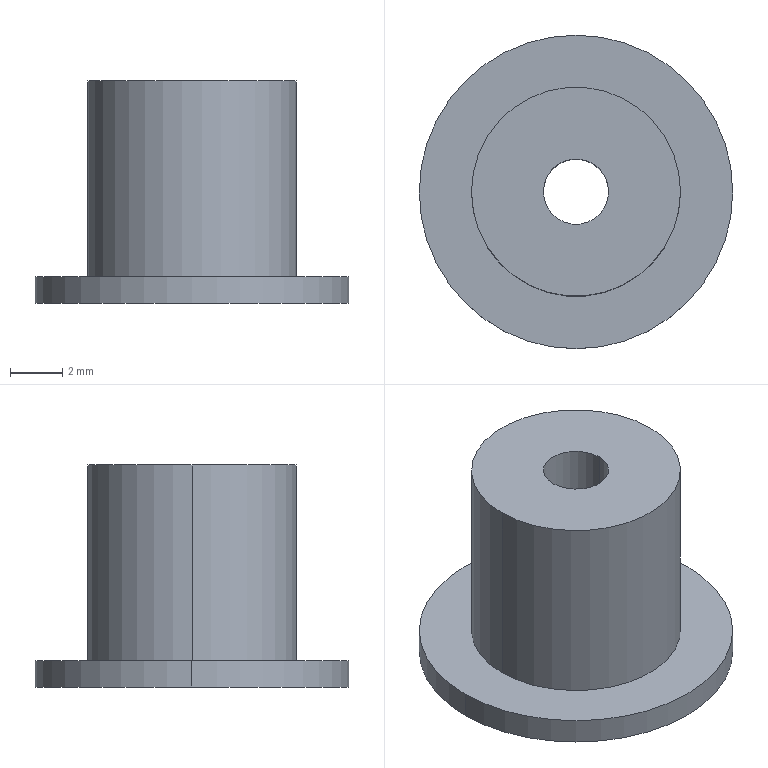Part | SolidWorks | features Extrusion 1, ICE 1 | 1 solid | 9 faces | box 12 x 12 x 8.5 mm | volume 448.364 mm3 | cylinder 6 | plane 3 | commonest cylinder face diameters 2.5 x2 8 x2 12 x2
STEP:
#1=CARTESIAN_POINT('',(6.,0.,-1.));
#2=VERTEX_POINT('',#1);
#3=CARTESIAN_POINT('',(-6.,0.,-1.));
#4=VERTEX_POINT('',#3);
#5=CARTESIAN_POINT('',(0.,0.,-1.));
#6=DIRECTION('',(0.,0.,1.));
#7=DIRECTION('',(1.,0.,0.));
#8=AXIS2_PLACEMENT_3D('',#5,#6,#7);
#9=CIRCLE('',#8,6.);
#10=EDGE_CURVE('',#2,#4,#9,.T.);
#11=ORIENTED_EDGE('',*,*,#10,.T.);
#12=CARTESIAN_POINT('',(-6.,0.,0.));
#13=VERTEX_POINT('',#12);
#14=CARTESIAN_POINT('',(-6.,0.,-1.));
#15=DIRECTION('',(0.,0.,1.));
#16=VECTOR('',#15,1000.);
#17=LINE('',#14,#16);
#18=EDGE_CURVE('',#4,#13,#17,.T.);
#19=ORIENTED_EDGE('',*,*,#18,.T.);
#20=CARTESIAN_POINT('',(6.,0.,0.));
#21=VERTEX_POINT('',#20);
#22=CARTESIAN_POINT('',(0.,0.,0.));
#23=DIRECTION('',(0.,0.,1.));
#24=DIRECTION('',(1.,0.,0.));
#25=AXIS2_PLACEMENT_3D('',#22,#23,#24);
#26=CIRCLE('',#25,6.);
#27=EDGE_CURVE('',#21,#13,#26,.T.);
#28=ORIENTED_EDGE('',*,*,#27,.F.);
#29=CARTESIAN_POINT('',(6.,0.,-1.));
#30=DIRECTION('',(0.,0.,1.));
#31=VECTOR('',#30,1000.);
#32=LINE('',#29,#31);
#33=EDGE_CURVE('',#2,#21,#32,.T.);
#34=ORIENTED_EDGE('',*,*,#33,.F.);
#35=EDGE_LOOP('',(#11,#19,#28,#34));
#36=FACE_OUTER_BOUND('',#35,.T.);
#37=CARTESIAN_POINT('',(0.,0.,-1.));
#38=DIRECTION('',(0.,0.,1.));
#39=DIRECTION('',(1.,0.,0.));
#40=AXIS2_PLACEMENT_3D('',#37,#38,#39);
#41=CYLINDRICAL_SURFACE('',#40,6.);
#42=ADVANCED_FACE('',(#36),#41,.T.);
#43=CARTESIAN_POINT('',(-1.25,0.,7.5));
#44=VERTEX_POINT('',#43);
#45=CARTESIAN_POINT('',(1.25,0.,7.5));
#46=VERTEX_POINT('',#45);
#47=CARTESIAN_POINT('',(0.,0.,7.5));
#48=DIRECTION('',(0.,0.,1.));
#49=DIRECTION('',(1.,0.,0.));
#50=AXIS2_PLACEMENT_3D('',#47,#48,#49);
#51=CIRCLE('',#50,1.25);
#52=EDGE_CURVE('',#44,#46,#51,.T.);
#53=ORIENTED_EDGE('',*,*,#52,.T.);
#54=CARTESIAN_POINT('',(1.25,0.,-1.));
#55=VERTEX_POINT('',#54);
#56=CARTESIAN_POINT('',(1.25,0.,7.5));
#57=DIRECTION('',(0.,0.,-1.));
#58=VECTOR('',#57,1000.);
#59=LINE('',#56,#58);
#60=EDGE_CURVE('',#46,#55,#59,.T.);
#61=ORIENTED_EDGE('',*,*,#60,.T.);
#62=CARTESIAN_POINT('',(-1.25,0.,-1.));
#63=VERTEX_POINT('',#62);
#64=CARTESIAN_POINT('',(0.,0.,-1.));
#65=DIRECTION('',(0.,0.,1.));
#66=DIRECTION('',(1.,0.,0.));
#67=AXIS2_PLACEMENT_3D('',#64,#65,#66);
#68=CIRCLE('',#67,1.25);
#69=EDGE_CURVE('',#63,#55,#68,.T.);
#70=ORIENTED_EDGE('',*,*,#69,.F.);
#71=CARTESIAN_POINT('',(-1.25,0.,7.5));
#72=DIRECTION('',(0.,0.,-1.));
#73=VECTOR('',#72,1000.);
#74=LINE('',#71,#73);
#75=EDGE_CURVE('',#44,#63,#74,.T.);
#76=ORIENTED_EDGE('',*,*,#75,.F.);
#77=EDGE_LOOP('',(#53,#61,#70,#76));
#78=FACE_OUTER_BOUND('',#77,.T.);
#79=CARTESIAN_POINT('',(0.,0.,7.5));
#80=DIRECTION('',(0.,0.,-1.));
#81=DIRECTION('',(-1.,0.,0.));
#82=AXIS2_PLACEMENT_3D('',#79,#80,#81);
#83=CYLINDRICAL_SURFACE('',#82,1.25);
#84=ADVANCED_FACE('',(#78),#83,.F.);
#85=CARTESIAN_POINT('',(4.,0.,7.5));
#86=VERTEX_POINT('',#85);
#87=CARTESIAN_POINT('',(-4.,0.,7.5));
#88=VERTEX_POINT('',#87);
#89=CARTESIAN_POINT('',(0.,0.,7.5));
#90=DIRECTION('',(0.,0.,1.));
#91=DIRECTION('',(1.,0.,0.));
#92=AXIS2_PLACEMENT_3D('',#89,#90,#91);
#93=CIRCLE('',#92,4.);
#94=EDGE_CURVE('',#86,#88,#93,.T.);
#95=ORIENTED_EDGE('',*,*,#94,.F.);
#96=CARTESIAN_POINT('',(4.,0.,0.));
#97=VERTEX_POINT('',#96);
#98=CARTESIAN_POINT('',(4.,0.,7.5));
#99=DIRECTION('',(0.,0.,-1.));
#100=VECTOR('',#99,1000.);
#101=LINE('',#98,#100);
#102=EDGE_CURVE('',#86,#97,#101,.T.);
#103=ORIENTED_EDGE('',*,*,#102,.T.);
#104=CARTESIAN_POINT('',(-4.,0.,0.));
#105=VERTEX_POINT('',#104);
#106=CARTESIAN_POINT('',(0.,0.,0.));
#107=DIRECTION('',(0.,0.,1.));
#108=DIRECTION('',(1.,0.,0.));
#109=AXIS2_PLACEMENT_3D('',#106,#107,#108);
#110=CIRCLE('',#109,4.);
#111=EDGE_CURVE('',#97,#105,#110,.T.);
#112=ORIENTED_EDGE('',*,*,#111,.T.);
#113=CARTESIAN_POINT('',(-4.,0.,7.5));
#114=DIRECTION('',(0.,0.,-1.));
#115=VECTOR('',#114,1000.);
#116=LINE('',#113,#115);
#117=EDGE_CURVE('',#88,#105,#116,.T.);
#118=ORIENTED_EDGE('',*,*,#117,.F.);
#119=EDGE_LOOP('',(#95,#103,#112,#118));
#120=FACE_OUTER_BOUND('',#119,.T.);
#121=CARTESIAN_POINT('',(0.,0.,7.5));
#122=DIRECTION('',(0.,0.,-1.));
#123=DIRECTION('',(-1.,0.,0.));
#124=AXIS2_PLACEMENT_3D('',#121,#122,#123);
#125=CYLINDRICAL_SURFACE('',#124,4.);
#126=ADVANCED_FACE('',(#120),#125,.T.);
#127=CARTESIAN_POINT('',(0.,0.,7.5));
#128=DIRECTION('',(0.,0.,1.));
#129=DIRECTION('',(1.,0.,0.));
#130=AXIS2_PLACEMENT_3D('',#127,#128,#129);
#131=CIRCLE('',#130,4.);
#132=EDGE_CURVE('',#88,#86,#131,.T.);
#133=ORIENTED_EDGE('',*,*,#132,.T.);
#134=ORIENTED_EDGE('',*,*,#94,.T.);
#135=EDGE_LOOP('',(#133,#134));
#136=FACE_OUTER_BOUND('',#135,.T.);
#137=ORIENTED_EDGE('',*,*,#52,.F.);
#138=CARTESIAN_POINT('',(0.,0.,7.5));
#139=DIRECTION('',(0.,0.,1.));
#140=DIRECTION('',(1.,0.,0.));
#141=AXIS2_PLACEMENT_3D('',#138,#139,#140);
#142=CIRCLE('',#141,1.25);
#143=EDGE_CURVE('',#46,#44,#142,.T.);
#144=ORIENTED_EDGE('',*,*,#143,.F.);
#145=EDGE_LOOP('',(#137,#144));
#146=FACE_BOUND('',#145,.T.);
#147=CARTESIAN_POINT('',(0.,0.,7.5));
#148=DIRECTION('',(0.,0.,1.));
#149=DIRECTION('',(1.,0.,0.));
#150=AXIS2_PLACEMENT_3D('',#147,#148,#149);
#151=PLANE('',#150);
#152=ADVANCED_FACE('',(#136,#146),#151,.T.);
#153=ORIENTED_EDGE('',*,*,#102,.F.);
#154=ORIENTED_EDGE('',*,*,#132,.F.);
#155=ORIENTED_EDGE('',*,*,#117,.T.);
#156=CARTESIAN_POINT('',(0.,0.,0.));
#157=DIRECTION('',(0.,0.,1.));
#158=DIRECTION('',(1.,0.,0.));
#159=AXIS2_PLACEMENT_3D('',#156,#157,#158);
#160=CIRCLE('',#159,4.);
#161=EDGE_CURVE('',#105,#97,#160,.T.);
#162=ORIENTED_EDGE('',*,*,#161,.T.);
#163=EDGE_LOOP('',(#153,#154,#155,#162));
#164=FACE_OUTER_BOUND('',#163,.T.);
#165=CARTESIAN_POINT('',(0.,0.,7.5));
#166=DIRECTION('',(0.,0.,-1.));
#167=DIRECTION('',(-1.,0.,0.));
#168=AXIS2_PLACEMENT_3D('',#165,#166,#167);
#169=CYLINDRICAL_SURFACE('',#168,4.);
#170=ADVANCED_FACE('',(#164),#169,.T.);
#171=ORIENTED_EDGE('',*,*,#60,.F.);
#172=ORIENTED_EDGE('',*,*,#143,.T.);
#173=ORIENTED_EDGE('',*,*,#75,.T.);
#174=CARTESIAN_POINT('',(0.,0.,-1.));
#175=DIRECTION('',(0.,0.,1.));
#176=DIRECTION('',(1.,0.,0.));
#177=AXIS2_PLACEMENT_3D('',#174,#175,#176);
#178=CIRCLE('',#177,1.25);
#179=EDGE_CURVE('',#55,#63,#178,.T.);
#180=ORIENTED_EDGE('',*,*,#179,.F.);
#181=EDGE_LOOP('',(#171,#172,#173,#180));
#182=FACE_OUTER_BOUND('',#181,.T.);
#183=CARTESIAN_POINT('',(0.,0.,7.5));
#184=DIRECTION('',(0.,0.,-1.));
#185=DIRECTION('',(-1.,0.,0.));
#186=AXIS2_PLACEMENT_3D('',#183,#184,#185);
#187=CYLINDRICAL_SURFACE('',#186,1.25);
#188=ADVANCED_FACE('',(#182),#187,.F.);
#189=ORIENTED_EDGE('',*,*,#18,.F.);
#190=CARTESIAN_POINT('',(0.,0.,-1.));
#191=DIRECTION('',(0.,0.,1.));
#192=DIRECTION('',(1.,0.,0.));
#193=AXIS2_PLACEMENT_3D('',#190,#191,#192);
#194=CIRCLE('',#193,6.);
#195=EDGE_CURVE('',#4,#2,#194,.T.);
#196=ORIENTED_EDGE('',*,*,#195,.T.);
#197=ORIENTED_EDGE('',*,*,#33,.T.);
#198=CARTESIAN_POINT('',(0.,0.,0.));
#199=DIRECTION('',(0.,0.,1.));
#200=DIRECTION('',(1.,0.,0.));
#201=AXIS2_PLACEMENT_3D('',#198,#199,#200);
#202=CIRCLE('',#201,6.);
#203=EDGE_CURVE('',#13,#21,#202,.T.);
#204=ORIENTED_EDGE('',*,*,#203,.F.);
#205=EDGE_LOOP('',(#189,#196,#197,#204));
#206=FACE_OUTER_BOUND('',#205,.T.);
#207=CARTESIAN_POINT('',(0.,0.,-1.));
#208=DIRECTION('',(0.,0.,1.));
#209=DIRECTION('',(1.,0.,0.));
#210=AXIS2_PLACEMENT_3D('',#207,#208,#209);
#211=CYLINDRICAL_SURFACE('',#210,6.);
#212=ADVANCED_FACE('',(#206),#211,.T.);
#213=ORIENTED_EDGE('',*,*,#69,.T.);
#214=ORIENTED_EDGE('',*,*,#179,.T.);
#215=EDGE_LOOP('',(#213,#214));
#216=FACE_BOUND('',#215,.T.);
#217=ORIENTED_EDGE('',*,*,#10,.F.);
#218=ORIENTED_EDGE('',*,*,#195,.F.);
#219=EDGE_LOOP('',(#217,#218));
#220=FACE_OUTER_BOUND('',#219,.T.);
#221=CARTESIAN_POINT('',(0.,0.,-1.));
#222=DIRECTION('',(0.,0.,1.));
#223=DIRECTION('',(1.,0.,0.));
#224=AXIS2_PLACEMENT_3D('',#221,#222,#223);
#225=PLANE('',#224);
#226=ADVANCED_FACE('',(#216,#220),#225,.F.);
#227=ORIENTED_EDGE('',*,*,#161,.F.);
#228=ORIENTED_EDGE('',*,*,#111,.F.);
#229=EDGE_LOOP('',(#227,#228));
#230=FACE_BOUND('',#229,.T.);
#231=ORIENTED_EDGE('',*,*,#27,.T.);
#232=ORIENTED_EDGE('',*,*,#203,.T.);
#233=EDGE_LOOP('',(#231,#232));
#234=FACE_OUTER_BOUND('',#233,.T.);
#235=CARTESIAN_POINT('',(0.,0.,0.));
#236=DIRECTION('',(0.,0.,1.));
#237=DIRECTION('',(1.,0.,0.));
#238=AXIS2_PLACEMENT_3D('',#235,#236,#237);
#239=PLANE('',#238);
#240=ADVANCED_FACE('',(#230,#234),#239,.T.);
#241=CLOSED_SHELL('',(#42,#84,#126,#152,#170,#188,#212,#226,#240));
#242=MANIFOLD_SOLID_BREP('',#241);
#243=CARTESIAN_POINT('',(0.,0.,0.));
#244=DIRECTION('',(0.,0.,1.));
#245=DIRECTION('',(1.,0.,0.));
#246=AXIS2_PLACEMENT_3D('',#243,#244,#245);
#247=(LENGTH_UNIT()NAMED_UNIT(*)SI_UNIT(.MILLI.,.METRE.));
#248=UNCERTAINTY_MEASURE_WITH_UNIT(LENGTH_MEASURE(0.00001),#247,'','');
#249=(NAMED_UNIT(*)PLANE_ANGLE_UNIT()SI_UNIT($,.RADIAN.));
#250=(NAMED_UNIT(*)SI_UNIT($,.STERADIAN.)SOLID_ANGLE_UNIT());
#251=(GEOMETRIC_REPRESENTATION_CONTEXT(3)GLOBAL_UNCERTAINTY_ASSIGNED_CONTEXT((#248))GLOBAL_UNIT_ASSIGNED_CONTEXT((#247,#249,#250))REPRESENTATION_CONTEXT('',''));
#252=ADVANCED_BREP_SHAPE_REPRESENTATION('',(#242,#246),#251);